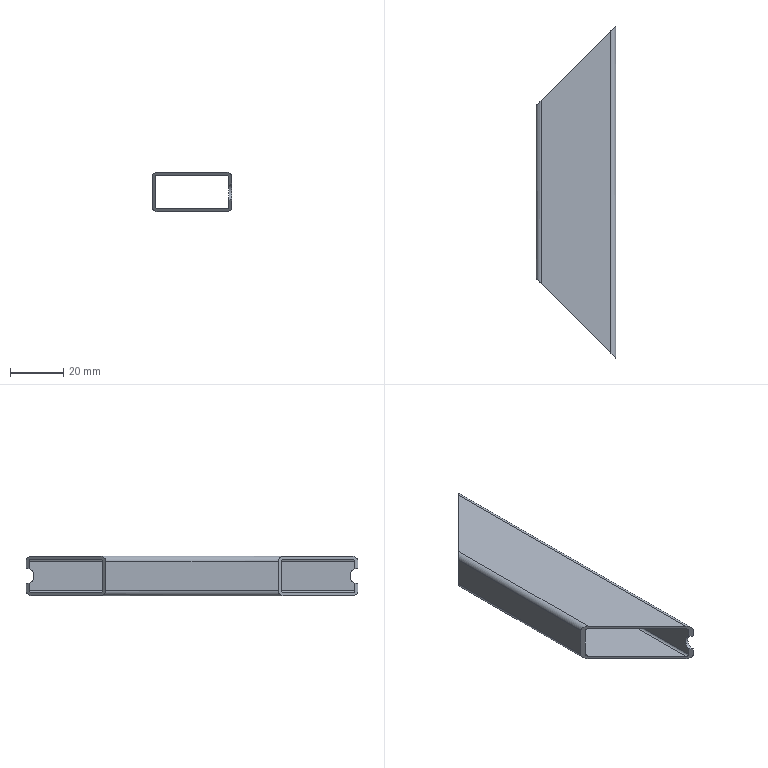Part | STEP file | 6150403 | 1 solid | 20 faces | box 30 x 125 x 15 mm | volume 9413 mm3 | cylinder 10 | plane 10 | commonest cylinder face diameters 1.6 x4 4 x4 6 x2
STEP:
#1=CARTESIAN_POINT('',(-13.,34.5,-7.5));
#2=VERTEX_POINT('',#1);
#3=CARTESIAN_POINT('',(-13.,-34.5,-7.5));
#4=VERTEX_POINT('',#3);
#5=CARTESIAN_POINT('',(-13.,62.5,-7.5));
#6=DIRECTION('',(0.,-1.,0.));
#7=VECTOR('',#6,1000.);
#8=LINE('',#5,#7);
#9=EDGE_CURVE('',#2,#4,#8,.T.);
#10=ORIENTED_EDGE('',*,*,#9,.T.);
#11=CARTESIAN_POINT('',(-15.,-32.5,-5.5));
#12=VERTEX_POINT('',#11);
#13=CARTESIAN_POINT('',(-13.,-34.5,-7.5));
#14=CARTESIAN_POINT('',(-14.172,-33.328,-7.5));
#15=CARTESIAN_POINT('',(-15.,-32.5,-6.672));
#16=CARTESIAN_POINT('',(-15.,-32.5,-5.5));
#17=(BOUNDED_CURVE()B_SPLINE_CURVE(3,(#13,#14,#15,#16),.UNSPECIFIED.,.F.,.F.)B_SPLINE_CURVE_WITH_KNOTS((4,4),(1.571,3.142),.UNSPECIFIED.)CURVE()GEOMETRIC_REPRESENTATION_ITEM()RATIONAL_B_SPLINE_CURVE((1.,0.8047,0.8047,1.))REPRESENTATION_ITEM(''));
#18=EDGE_CURVE('',#4,#12,#17,.T.);
#19=ORIENTED_EDGE('',*,*,#18,.T.);
#20=CARTESIAN_POINT('',(-15.,32.5,-5.5));
#21=VERTEX_POINT('',#20);
#22=CARTESIAN_POINT('',(-15.,62.5,-5.5));
#23=DIRECTION('',(0.,-1.,0.));
#24=VECTOR('',#23,1000.);
#25=LINE('',#22,#24);
#26=EDGE_CURVE('',#21,#12,#25,.T.);
#27=ORIENTED_EDGE('',*,*,#26,.F.);
#28=CARTESIAN_POINT('',(-15.,32.5,-5.5));
#29=CARTESIAN_POINT('',(-15.,32.5,-6.672));
#30=CARTESIAN_POINT('',(-14.172,33.328,-7.5));
#31=CARTESIAN_POINT('',(-13.,34.5,-7.5));
#32=(BOUNDED_CURVE()B_SPLINE_CURVE(3,(#28,#29,#30,#31),.UNSPECIFIED.,.F.,.F.)B_SPLINE_CURVE_WITH_KNOTS((4,4),(0.,1.571),.UNSPECIFIED.)CURVE()GEOMETRIC_REPRESENTATION_ITEM()RATIONAL_B_SPLINE_CURVE((1.,0.8047,0.8047,1.))REPRESENTATION_ITEM(''));
#33=EDGE_CURVE('',#21,#2,#32,.T.);
#34=ORIENTED_EDGE('',*,*,#33,.T.);
#35=EDGE_LOOP('',(#10,#19,#27,#34));
#36=FACE_OUTER_BOUND('',#35,.T.);
#37=CARTESIAN_POINT('',(-13.,62.5,-5.5));
#38=DIRECTION('',(0.,-1.,0.));
#39=DIRECTION('',(0.,0.,-1.));
#40=AXIS2_PLACEMENT_3D('',#37,#38,#39);
#41=CYLINDRICAL_SURFACE('',#40,2.);
#42=ADVANCED_FACE('',(#36),#41,.T.);
#43=ORIENTED_EDGE('',*,*,#26,.T.);
#44=CARTESIAN_POINT('',(-15.,-32.5,5.5));
#45=VERTEX_POINT('',#44);
#46=CARTESIAN_POINT('',(-15.,-32.5,192.5));
#47=DIRECTION('',(0.,0.,-1.));
#48=VECTOR('',#47,1000.);
#49=LINE('',#46,#48);
#50=EDGE_CURVE('',#45,#12,#49,.T.);
#51=ORIENTED_EDGE('',*,*,#50,.F.);
#52=CARTESIAN_POINT('',(-15.,32.5,5.5));
#53=VERTEX_POINT('',#52);
#54=CARTESIAN_POINT('',(-15.,62.5,5.5));
#55=DIRECTION('',(0.,-1.,0.));
#56=VECTOR('',#55,1000.);
#57=LINE('',#54,#56);
#58=EDGE_CURVE('',#53,#45,#57,.T.);
#59=ORIENTED_EDGE('',*,*,#58,.F.);
#60=CARTESIAN_POINT('',(-15.,32.5,192.5));
#61=DIRECTION('',(0.,0.,-1.));
#62=VECTOR('',#61,1000.);
#63=LINE('',#60,#62);
#64=EDGE_CURVE('',#53,#21,#63,.T.);
#65=ORIENTED_EDGE('',*,*,#64,.T.);
#66=EDGE_LOOP('',(#43,#51,#59,#65));
#67=FACE_OUTER_BOUND('',#66,.T.);
#68=CARTESIAN_POINT('',(-15.,62.5,-5.5));
#69=DIRECTION('',(1.,0.,0.));
#70=DIRECTION('',(0.,0.,-1.));
#71=AXIS2_PLACEMENT_3D('',#68,#69,#70);
#72=PLANE('',#71);
#73=ADVANCED_FACE('',(#67),#72,.F.);
#74=ORIENTED_EDGE('',*,*,#58,.T.);
#75=CARTESIAN_POINT('',(-13.,-34.5,7.5));
#76=VERTEX_POINT('',#75);
#77=CARTESIAN_POINT('',(-15.,-32.5,5.5));
#78=CARTESIAN_POINT('',(-15.,-32.5,6.672));
#79=CARTESIAN_POINT('',(-14.172,-33.328,7.5));
#80=CARTESIAN_POINT('',(-13.,-34.5,7.5));
#81=(BOUNDED_CURVE()B_SPLINE_CURVE(3,(#77,#78,#79,#80),.UNSPECIFIED.,.F.,.F.)B_SPLINE_CURVE_WITH_KNOTS((4,4),(3.142,4.712),.UNSPECIFIED.)CURVE()GEOMETRIC_REPRESENTATION_ITEM()RATIONAL_B_SPLINE_CURVE((1.,0.8047,0.8047,1.))REPRESENTATION_ITEM(''));
#82=EDGE_CURVE('',#45,#76,#81,.T.);
#83=ORIENTED_EDGE('',*,*,#82,.T.);
#84=CARTESIAN_POINT('',(-13.,34.5,7.5));
#85=VERTEX_POINT('',#84);
#86=CARTESIAN_POINT('',(-13.,62.5,7.5));
#87=DIRECTION('',(0.,-1.,0.));
#88=VECTOR('',#87,1000.);
#89=LINE('',#86,#88);
#90=EDGE_CURVE('',#85,#76,#89,.T.);
#91=ORIENTED_EDGE('',*,*,#90,.F.);
#92=CARTESIAN_POINT('',(-13.,34.5,7.5));
#93=CARTESIAN_POINT('',(-14.172,33.328,7.5));
#94=CARTESIAN_POINT('',(-15.,32.5,6.672));
#95=CARTESIAN_POINT('',(-15.,32.5,5.5));
#96=(BOUNDED_CURVE()B_SPLINE_CURVE(3,(#92,#93,#94,#95),.UNSPECIFIED.,.F.,.F.)B_SPLINE_CURVE_WITH_KNOTS((4,4),(4.712,6.283),.UNSPECIFIED.)CURVE()GEOMETRIC_REPRESENTATION_ITEM()RATIONAL_B_SPLINE_CURVE((1.,0.8047,0.8047,1.))REPRESENTATION_ITEM(''));
#97=EDGE_CURVE('',#85,#53,#96,.T.);
#98=ORIENTED_EDGE('',*,*,#97,.T.);
#99=EDGE_LOOP('',(#74,#83,#91,#98));
#100=FACE_OUTER_BOUND('',#99,.T.);
#101=CARTESIAN_POINT('',(-13.,62.5,5.5));
#102=DIRECTION('',(0.,-1.,0.));
#103=DIRECTION('',(0.,0.,-1.));
#104=AXIS2_PLACEMENT_3D('',#101,#102,#103);
#105=CYLINDRICAL_SURFACE('',#104,2.);
#106=ADVANCED_FACE('',(#100),#105,.T.);
#107=ORIENTED_EDGE('',*,*,#90,.T.);
#108=CARTESIAN_POINT('',(13.,-60.5,7.5));
#109=VERTEX_POINT('',#108);
#110=CARTESIAN_POINT('',(-61.5,14.,7.5));
#111=DIRECTION('',(0.7071,-0.7071,0.));
#112=VECTOR('',#111,1000.);
#113=LINE('',#110,#112);
#114=EDGE_CURVE('',#76,#109,#113,.T.);
#115=ORIENTED_EDGE('',*,*,#114,.T.);
#116=CARTESIAN_POINT('',(13.,60.5,7.5));
#117=VERTEX_POINT('',#116);
#118=CARTESIAN_POINT('',(13.,62.5,7.5));
#119=DIRECTION('',(0.,-1.,0.));
#120=VECTOR('',#119,1000.);
#121=LINE('',#118,#120);
#122=EDGE_CURVE('',#117,#109,#121,.T.);
#123=ORIENTED_EDGE('',*,*,#122,.F.);
#124=CARTESIAN_POINT('',(1.,48.5,7.5));
#125=DIRECTION('',(-0.7071,-0.7071,0.));
#126=VECTOR('',#125,1000.);
#127=LINE('',#124,#126);
#128=EDGE_CURVE('',#117,#85,#127,.T.);
#129=ORIENTED_EDGE('',*,*,#128,.T.);
#130=EDGE_LOOP('',(#107,#115,#123,#129));
#131=FACE_OUTER_BOUND('',#130,.T.);
#132=CARTESIAN_POINT('',(-13.,62.5,7.5));
#133=DIRECTION('',(0.,0.,-1.));
#134=DIRECTION('',(-1.,0.,0.));
#135=AXIS2_PLACEMENT_3D('',#132,#133,#134);
#136=PLANE('',#135);
#137=ADVANCED_FACE('',(#131),#136,.F.);
#138=ORIENTED_EDGE('',*,*,#122,.T.);
#139=CARTESIAN_POINT('',(15.,-62.5,5.5));
#140=VERTEX_POINT('',#139);
#141=CARTESIAN_POINT('',(13.,-60.5,7.5));
#142=CARTESIAN_POINT('',(14.172,-61.672,7.5));
#143=CARTESIAN_POINT('',(15.,-62.5,6.672));
#144=CARTESIAN_POINT('',(15.,-62.5,5.5));
#145=(BOUNDED_CURVE()B_SPLINE_CURVE(3,(#141,#142,#143,#144),.UNSPECIFIED.,.F.,.F.)B_SPLINE_CURVE_WITH_KNOTS((4,4),(4.712,6.283),.UNSPECIFIED.)CURVE()GEOMETRIC_REPRESENTATION_ITEM()RATIONAL_B_SPLINE_CURVE((1.,0.8047,0.8047,1.))REPRESENTATION_ITEM(''));
#146=EDGE_CURVE('',#109,#140,#145,.T.);
#147=ORIENTED_EDGE('',*,*,#146,.T.);
#148=CARTESIAN_POINT('',(15.,62.5,5.5));
#149=VERTEX_POINT('',#148);
#150=CARTESIAN_POINT('',(15.,62.5,5.5));
#151=DIRECTION('',(0.,-1.,0.));
#152=VECTOR('',#151,1000.);
#153=LINE('',#150,#152);
#154=EDGE_CURVE('',#149,#140,#153,.T.);
#155=ORIENTED_EDGE('',*,*,#154,.F.);
#156=CARTESIAN_POINT('',(15.,62.5,5.5));
#157=CARTESIAN_POINT('',(15.,62.5,6.672));
#158=CARTESIAN_POINT('',(14.172,61.672,7.5));
#159=CARTESIAN_POINT('',(13.,60.5,7.5));
#160=(BOUNDED_CURVE()B_SPLINE_CURVE(3,(#156,#157,#158,#159),.UNSPECIFIED.,.F.,.F.)B_SPLINE_CURVE_WITH_KNOTS((4,4),(3.142,4.712),.UNSPECIFIED.)CURVE()GEOMETRIC_REPRESENTATION_ITEM()RATIONAL_B_SPLINE_CURVE((1.,0.8047,0.8047,1.))REPRESENTATION_ITEM(''));
#161=EDGE_CURVE('',#149,#117,#160,.T.);
#162=ORIENTED_EDGE('',*,*,#161,.T.);
#163=EDGE_LOOP('',(#138,#147,#155,#162));
#164=FACE_OUTER_BOUND('',#163,.T.);
#165=CARTESIAN_POINT('',(13.,62.5,5.5));
#166=DIRECTION('',(0.,-1.,0.));
#167=DIRECTION('',(0.,0.,-1.));
#168=AXIS2_PLACEMENT_3D('',#165,#166,#167);
#169=CYLINDRICAL_SURFACE('',#168,2.);
#170=ADVANCED_FACE('',(#164),#169,.T.);
#171=CARTESIAN_POINT('',(15.,-62.5,3.));
#172=VERTEX_POINT('',#171);
#173=CARTESIAN_POINT('',(15.,-62.5,-5.5));
#174=DIRECTION('',(0.,0.,-1.));
#175=VECTOR('',#174,1000.);
#176=LINE('',#173,#175);
#177=EDGE_CURVE('',#140,#172,#176,.T.);
#178=ORIENTED_EDGE('',*,*,#177,.T.);
#179=CARTESIAN_POINT('',(15.,-62.5,-3.));
#180=VERTEX_POINT('',#179);
#181=CARTESIAN_POINT('',(15.,-62.5,0.));
#182=DIRECTION('',(1.,0.,0.));
#183=DIRECTION('',(0.,0.,-1.));
#184=AXIS2_PLACEMENT_3D('',#181,#182,#183);
#185=CIRCLE('',#184,3.);
#186=EDGE_CURVE('',#180,#172,#185,.T.);
#187=ORIENTED_EDGE('',*,*,#186,.F.);
#188=CARTESIAN_POINT('',(15.,-62.5,-5.5));
#189=VERTEX_POINT('',#188);
#190=CARTESIAN_POINT('',(15.,-62.5,-5.5));
#191=DIRECTION('',(0.,0.,-1.));
#192=VECTOR('',#191,1000.);
#193=LINE('',#190,#192);
#194=EDGE_CURVE('',#180,#189,#193,.T.);
#195=ORIENTED_EDGE('',*,*,#194,.T.);
#196=CARTESIAN_POINT('',(15.,62.5,-5.5));
#197=VERTEX_POINT('',#196);
#198=CARTESIAN_POINT('',(15.,62.5,-5.5));
#199=DIRECTION('',(0.,-1.,0.));
#200=VECTOR('',#199,1000.);
#201=LINE('',#198,#200);
#202=EDGE_CURVE('',#197,#189,#201,.T.);
#203=ORIENTED_EDGE('',*,*,#202,.F.);
#204=CARTESIAN_POINT('',(15.,62.5,-3.));
#205=VERTEX_POINT('',#204);
#206=CARTESIAN_POINT('',(15.,62.5,-5.5));
#207=DIRECTION('',(0.,0.,-1.));
#208=VECTOR('',#207,1000.);
#209=LINE('',#206,#208);
#210=EDGE_CURVE('',#205,#197,#209,.T.);
#211=ORIENTED_EDGE('',*,*,#210,.F.);
#212=CARTESIAN_POINT('',(15.,62.5,3.));
#213=VERTEX_POINT('',#212);
#214=CARTESIAN_POINT('',(15.,62.5,0.));
#215=DIRECTION('',(1.,0.,0.));
#216=DIRECTION('',(0.,0.,-1.));
#217=AXIS2_PLACEMENT_3D('',#214,#215,#216);
#218=CIRCLE('',#217,3.);
#219=EDGE_CURVE('',#213,#205,#218,.T.);
#220=ORIENTED_EDGE('',*,*,#219,.F.);
#221=CARTESIAN_POINT('',(15.,62.5,-5.5));
#222=DIRECTION('',(0.,0.,-1.));
#223=VECTOR('',#222,1000.);
#224=LINE('',#221,#223);
#225=EDGE_CURVE('',#149,#213,#224,.T.);
#226=ORIENTED_EDGE('',*,*,#225,.F.);
#227=ORIENTED_EDGE('',*,*,#154,.T.);
#228=EDGE_LOOP('',(#178,#187,#195,#203,#211,#220,#226,#227));
#229=FACE_OUTER_BOUND('',#228,.T.);
#230=CARTESIAN_POINT('',(15.,62.5,-5.5));
#231=DIRECTION('',(-1.,0.,0.));
#232=DIRECTION('',(0.,0.,1.));
#233=AXIS2_PLACEMENT_3D('',#230,#231,#232);
#234=PLANE('',#233);
#235=ADVANCED_FACE('',(#229),#234,.F.);
#236=ORIENTED_EDGE('',*,*,#202,.T.);
#237=CARTESIAN_POINT('',(13.,-60.5,-7.5));
#238=VERTEX_POINT('',#237);
#239=CARTESIAN_POINT('',(15.,-62.5,-5.5));
#240=CARTESIAN_POINT('',(15.,-62.5,-6.672));
#241=CARTESIAN_POINT('',(14.172,-61.672,-7.5));
#242=CARTESIAN_POINT('',(13.,-60.5,-7.5));
#243=(BOUNDED_CURVE()B_SPLINE_CURVE(3,(#239,#240,#241,#242),.UNSPECIFIED.,.F.,.F.)B_SPLINE_CURVE_WITH_KNOTS((4,4),(0.,1.571),.UNSPECIFIED.)CURVE()GEOMETRIC_REPRESENTATION_ITEM()RATIONAL_B_SPLINE_CURVE((1.,0.8047,0.8047,1.))REPRESENTATION_ITEM(''));
#244=EDGE_CURVE('',#189,#238,#243,.T.);
#245=ORIENTED_EDGE('',*,*,#244,.T.);
#246=CARTESIAN_POINT('',(13.,60.5,-7.5));
#247=VERTEX_POINT('',#246);
#248=CARTESIAN_POINT('',(13.,62.5,-7.5));
#249=DIRECTION('',(0.,-1.,0.));
#250=VECTOR('',#249,1000.);
#251=LINE('',#248,#250);
#252=EDGE_CURVE('',#247,#238,#251,.T.);
#253=ORIENTED_EDGE('',*,*,#252,.F.);
#254=CARTESIAN_POINT('',(13.,60.5,-7.5));
#255=CARTESIAN_POINT('',(14.172,61.672,-7.5));
#256=CARTESIAN_POINT('',(15.,62.5,-6.672));
#257=CARTESIAN_POINT('',(15.,62.5,-5.5));
#258=(BOUNDED_CURVE()B_SPLINE_CURVE(3,(#254,#255,#256,#257),.UNSPECIFIED.,.F.,.F.)B_SPLINE_CURVE_WITH_KNOTS((4,4),(1.571,3.142),.UNSPECIFIED.)CURVE()GEOMETRIC_REPRESENTATION_ITEM()RATIONAL_B_SPLINE_CURVE((1.,0.8047,0.8047,1.))REPRESENTATION_ITEM(''));
#259=EDGE_CURVE('',#247,#197,#258,.T.);
#260=ORIENTED_EDGE('',*,*,#259,.T.);
#261=EDGE_LOOP('',(#236,#245,#253,#260));
#262=FACE_OUTER_BOUND('',#261,.T.);
#263=CARTESIAN_POINT('',(13.,62.5,-5.5));
#264=DIRECTION('',(0.,-1.,0.));
#265=DIRECTION('',(0.,0.,-1.));
#266=AXIS2_PLACEMENT_3D('',#263,#264,#265);
#267=CYLINDRICAL_SURFACE('',#266,2.);
#268=ADVANCED_FACE('',(#262),#267,.T.);
#269=ORIENTED_EDGE('',*,*,#252,.T.);
#270=CARTESIAN_POINT('',(15.,-62.5,-7.5));
#271=DIRECTION('',(0.7071,-0.7071,0.));
#272=VECTOR('',#271,1000.);
#273=LINE('',#270,#272);
#274=EDGE_CURVE('',#4,#238,#273,.T.);
#275=ORIENTED_EDGE('',*,*,#274,.F.);
#276=ORIENTED_EDGE('',*,*,#9,.F.);
#277=CARTESIAN_POINT('',(15.,62.5,-7.5));
#278=DIRECTION('',(-0.7071,-0.7071,0.));
#279=VECTOR('',#278,1000.);
#280=LINE('',#277,#279);
#281=EDGE_CURVE('',#247,#2,#280,.T.);
#282=ORIENTED_EDGE('',*,*,#281,.F.);
#283=EDGE_LOOP('',(#269,#275,#276,#282));
#284=FACE_OUTER_BOUND('',#283,.T.);
#285=CARTESIAN_POINT('',(-13.,62.5,-7.5));
#286=DIRECTION('',(0.,0.,1.));
#287=DIRECTION('',(1.,0.,0.));
#288=AXIS2_PLACEMENT_3D('',#285,#286,#287);
#289=PLANE('',#288);
#290=ADVANCED_FACE('',(#284),#289,.F.);
#291=CARTESIAN_POINT('',(13.8,-61.3,-5.5));
#292=VERTEX_POINT('',#291);
#293=CARTESIAN_POINT('',(13.,-60.5,-6.3));
#294=VERTEX_POINT('',#293);
#295=CARTESIAN_POINT('',(13.8,-61.3,-5.5));
#296=CARTESIAN_POINT('',(13.8,-61.3,-5.969));
#297=CARTESIAN_POINT('',(13.469,-60.969,-6.3));
#298=CARTESIAN_POINT('',(13.,-60.5,-6.3));
#299=(BOUNDED_CURVE()B_SPLINE_CURVE(3,(#295,#296,#297,#298),.UNSPECIFIED.,.F.,.F.)B_SPLINE_CURVE_WITH_KNOTS((4,4),(0.,1.571),.UNSPECIFIED.)CURVE()GEOMETRIC_REPRESENTATION_ITEM()RATIONAL_B_SPLINE_CURVE((1.,0.8047,0.8047,1.))REPRESENTATION_ITEM(''));
#300=EDGE_CURVE('',#292,#294,#299,.T.);
#301=ORIENTED_EDGE('',*,*,#300,.F.);
#302=CARTESIAN_POINT('',(13.8,61.3,-5.5));
#303=VERTEX_POINT('',#302);
#304=CARTESIAN_POINT('',(13.8,62.5,-5.5));
#305=DIRECTION('',(0.,-1.,0.));
#306=VECTOR('',#305,1000.);
#307=LINE('',#304,#306);
#308=EDGE_CURVE('',#303,#292,#307,.T.);
#309=ORIENTED_EDGE('',*,*,#308,.F.);
#310=CARTESIAN_POINT('',(13.,60.5,-6.3));
#311=VERTEX_POINT('',#310);
#312=CARTESIAN_POINT('',(13.,60.5,-6.3));
#313=CARTESIAN_POINT('',(13.469,60.969,-6.3));
#314=CARTESIAN_POINT('',(13.8,61.3,-5.969));
#315=CARTESIAN_POINT('',(13.8,61.3,-5.5));
#316=(BOUNDED_CURVE()B_SPLINE_CURVE(3,(#312,#313,#314,#315),.UNSPECIFIED.,.F.,.F.)B_SPLINE_CURVE_WITH_KNOTS((4,4),(1.571,3.142),.UNSPECIFIED.)CURVE()GEOMETRIC_REPRESENTATION_ITEM()RATIONAL_B_SPLINE_CURVE((1.,0.8047,0.8047,1.))REPRESENTATION_ITEM(''));
#317=EDGE_CURVE('',#311,#303,#316,.T.);
#318=ORIENTED_EDGE('',*,*,#317,.F.);
#319=CARTESIAN_POINT('',(13.,62.5,-6.3));
#320=DIRECTION('',(0.,-1.,0.));
#321=VECTOR('',#320,1000.);
#322=LINE('',#319,#321);
#323=EDGE_CURVE('',#311,#294,#322,.T.);
#324=ORIENTED_EDGE('',*,*,#323,.T.);
#325=EDGE_LOOP('',(#301,#309,#318,#324));
#326=FACE_OUTER_BOUND('',#325,.T.);
#327=CARTESIAN_POINT('',(13.,62.5,-5.5));
#328=DIRECTION('',(0.,-1.,0.));
#329=DIRECTION('',(0.,0.,-1.));
#330=AXIS2_PLACEMENT_3D('',#327,#328,#329);
#331=CYLINDRICAL_SURFACE('',#330,0.8);
#332=ADVANCED_FACE('',(#326),#331,.F.);
#333=CARTESIAN_POINT('',(-13.,-34.5,-6.3));
#334=VERTEX_POINT('',#333);
#335=CARTESIAN_POINT('',(-61.5,14.,-6.3));
#336=DIRECTION('',(-0.7071,0.7071,0.));
#337=VECTOR('',#336,1000.);
#338=LINE('',#335,#337);
#339=EDGE_CURVE('',#294,#334,#338,.T.);
#340=ORIENTED_EDGE('',*,*,#339,.F.);
#341=ORIENTED_EDGE('',*,*,#323,.F.);
#342=CARTESIAN_POINT('',(-13.,34.5,-6.3));
#343=VERTEX_POINT('',#342);
#344=CARTESIAN_POINT('',(1.,48.5,-6.3));
#345=DIRECTION('',(0.7071,0.7071,0.));
#346=VECTOR('',#345,1000.);
#347=LINE('',#344,#346);
#348=EDGE_CURVE('',#343,#311,#347,.T.);
#349=ORIENTED_EDGE('',*,*,#348,.F.);
#350=CARTESIAN_POINT('',(-13.,62.5,-6.3));
#351=DIRECTION('',(0.,-1.,0.));
#352=VECTOR('',#351,1000.);
#353=LINE('',#350,#352);
#354=EDGE_CURVE('',#343,#334,#353,.T.);
#355=ORIENTED_EDGE('',*,*,#354,.T.);
#356=EDGE_LOOP('',(#340,#341,#349,#355));
#357=FACE_OUTER_BOUND('',#356,.T.);
#358=CARTESIAN_POINT('',(-13.,62.5,-6.3));
#359=DIRECTION('',(0.,0.,1.));
#360=DIRECTION('',(1.,0.,0.));
#361=AXIS2_PLACEMENT_3D('',#358,#359,#360);
#362=PLANE('',#361);
#363=ADVANCED_FACE('',(#357),#362,.T.);
#364=CARTESIAN_POINT('',(-13.8,-33.7,-5.5));
#365=VERTEX_POINT('',#364);
#366=CARTESIAN_POINT('',(-13.,-34.5,-6.3));
#367=CARTESIAN_POINT('',(-13.469,-34.031,-6.3));
#368=CARTESIAN_POINT('',(-13.8,-33.7,-5.969));
#369=CARTESIAN_POINT('',(-13.8,-33.7,-5.5));
#370=(BOUNDED_CURVE()B_SPLINE_CURVE(3,(#366,#367,#368,#369),.UNSPECIFIED.,.F.,.F.)B_SPLINE_CURVE_WITH_KNOTS((4,4),(1.571,3.142),.UNSPECIFIED.)CURVE()GEOMETRIC_REPRESENTATION_ITEM()RATIONAL_B_SPLINE_CURVE((1.,0.8047,0.8047,1.))REPRESENTATION_ITEM(''));
#371=EDGE_CURVE('',#334,#365,#370,.T.);
#372=ORIENTED_EDGE('',*,*,#371,.F.);
#373=ORIENTED_EDGE('',*,*,#354,.F.);
#374=CARTESIAN_POINT('',(-13.8,33.7,-5.5));
#375=VERTEX_POINT('',#374);
#376=CARTESIAN_POINT('',(-13.8,33.7,-5.5));
#377=CARTESIAN_POINT('',(-13.8,33.7,-5.969));
#378=CARTESIAN_POINT('',(-13.469,34.031,-6.3));
#379=CARTESIAN_POINT('',(-13.,34.5,-6.3));
#380=(BOUNDED_CURVE()B_SPLINE_CURVE(3,(#376,#377,#378,#379),.UNSPECIFIED.,.F.,.F.)B_SPLINE_CURVE_WITH_KNOTS((4,4),(0.,1.571),.UNSPECIFIED.)CURVE()GEOMETRIC_REPRESENTATION_ITEM()RATIONAL_B_SPLINE_CURVE((1.,0.8047,0.8047,1.))REPRESENTATION_ITEM(''));
#381=EDGE_CURVE('',#375,#343,#380,.T.);
#382=ORIENTED_EDGE('',*,*,#381,.F.);
#383=CARTESIAN_POINT('',(-13.8,62.5,-5.5));
#384=DIRECTION('',(0.,-1.,0.));
#385=VECTOR('',#384,1000.);
#386=LINE('',#383,#385);
#387=EDGE_CURVE('',#375,#365,#386,.T.);
#388=ORIENTED_EDGE('',*,*,#387,.T.);
#389=EDGE_LOOP('',(#372,#373,#382,#388));
#390=FACE_OUTER_BOUND('',#389,.T.);
#391=CARTESIAN_POINT('',(-13.,62.5,-5.5));
#392=DIRECTION('',(0.,-1.,0.));
#393=DIRECTION('',(0.,0.,-1.));
#394=AXIS2_PLACEMENT_3D('',#391,#392,#393);
#395=CYLINDRICAL_SURFACE('',#394,0.8);
#396=ADVANCED_FACE('',(#390),#395,.F.);
#397=CARTESIAN_POINT('',(-13.8,-33.7,5.5));
#398=VERTEX_POINT('',#397);
#399=CARTESIAN_POINT('',(-13.8,-33.7,-5.5));
#400=DIRECTION('',(0.,0.,1.));
#401=VECTOR('',#400,1000.);
#402=LINE('',#399,#401);
#403=EDGE_CURVE('',#365,#398,#402,.T.);
#404=ORIENTED_EDGE('',*,*,#403,.F.);
#405=ORIENTED_EDGE('',*,*,#387,.F.);
#406=CARTESIAN_POINT('',(-13.8,33.7,5.5));
#407=VERTEX_POINT('',#406);
#408=CARTESIAN_POINT('',(-13.8,33.7,-5.5));
#409=DIRECTION('',(0.,0.,-1.));
#410=VECTOR('',#409,1000.);
#411=LINE('',#408,#410);
#412=EDGE_CURVE('',#407,#375,#411,.T.);
#413=ORIENTED_EDGE('',*,*,#412,.F.);
#414=CARTESIAN_POINT('',(-13.8,62.5,5.5));
#415=DIRECTION('',(0.,-1.,0.));
#416=VECTOR('',#415,1000.);
#417=LINE('',#414,#416);
#418=EDGE_CURVE('',#407,#398,#417,.T.);
#419=ORIENTED_EDGE('',*,*,#418,.T.);
#420=EDGE_LOOP('',(#404,#405,#413,#419));
#421=FACE_OUTER_BOUND('',#420,.T.);
#422=CARTESIAN_POINT('',(-13.8,62.5,-5.5));
#423=DIRECTION('',(1.,0.,0.));
#424=DIRECTION('',(0.,0.,-1.));
#425=AXIS2_PLACEMENT_3D('',#422,#423,#424);
#426=PLANE('',#425);
#427=ADVANCED_FACE('',(#421),#426,.T.);
#428=CARTESIAN_POINT('',(-13.,-34.5,6.3));
#429=VERTEX_POINT('',#428);
#430=CARTESIAN_POINT('',(-13.8,-33.7,5.5));
#431=CARTESIAN_POINT('',(-13.8,-33.7,5.969));
#432=CARTESIAN_POINT('',(-13.469,-34.031,6.3));
#433=CARTESIAN_POINT('',(-13.,-34.5,6.3));
#434=(BOUNDED_CURVE()B_SPLINE_CURVE(3,(#430,#431,#432,#433),.UNSPECIFIED.,.F.,.F.)B_SPLINE_CURVE_WITH_KNOTS((4,4),(3.142,4.712),.UNSPECIFIED.)CURVE()GEOMETRIC_REPRESENTATION_ITEM()RATIONAL_B_SPLINE_CURVE((1.,0.8047,0.8047,1.))REPRESENTATION_ITEM(''));
#435=EDGE_CURVE('',#398,#429,#434,.T.);
#436=ORIENTED_EDGE('',*,*,#435,.F.);
#437=ORIENTED_EDGE('',*,*,#418,.F.);
#438=CARTESIAN_POINT('',(-13.,34.5,6.3));
#439=VERTEX_POINT('',#438);
#440=CARTESIAN_POINT('',(-13.,34.5,6.3));
#441=CARTESIAN_POINT('',(-13.469,34.031,6.3));
#442=CARTESIAN_POINT('',(-13.8,33.7,5.969));
#443=CARTESIAN_POINT('',(-13.8,33.7,5.5));
#444=(BOUNDED_CURVE()B_SPLINE_CURVE(3,(#440,#441,#442,#443),.UNSPECIFIED.,.F.,.F.)B_SPLINE_CURVE_WITH_KNOTS((4,4),(4.712,6.283),.UNSPECIFIED.)CURVE()GEOMETRIC_REPRESENTATION_ITEM()RATIONAL_B_SPLINE_CURVE((1.,0.8047,0.8047,1.))REPRESENTATION_ITEM(''));
#445=EDGE_CURVE('',#439,#407,#444,.T.);
#446=ORIENTED_EDGE('',*,*,#445,.F.);
#447=CARTESIAN_POINT('',(-13.,62.5,6.3));
#448=DIRECTION('',(0.,-1.,0.));
#449=VECTOR('',#448,1000.);
#450=LINE('',#447,#449);
#451=EDGE_CURVE('',#439,#429,#450,.T.);
#452=ORIENTED_EDGE('',*,*,#451,.T.);
#453=EDGE_LOOP('',(#436,#437,#446,#452));
#454=FACE_OUTER_BOUND('',#453,.T.);
#455=CARTESIAN_POINT('',(-13.,62.5,5.5));
#456=DIRECTION('',(0.,-1.,0.));
#457=DIRECTION('',(0.,0.,-1.));
#458=AXIS2_PLACEMENT_3D('',#455,#456,#457);
#459=CYLINDRICAL_SURFACE('',#458,0.8);
#460=ADVANCED_FACE('',(#454),#459,.F.);
#461=CARTESIAN_POINT('',(13.,-60.5,6.3));
#462=VERTEX_POINT('',#461);
#463=CARTESIAN_POINT('',(-61.5,14.,6.3));
#464=DIRECTION('',(0.7071,-0.7071,0.));
#465=VECTOR('',#464,1000.);
#466=LINE('',#463,#465);
#467=EDGE_CURVE('',#429,#462,#466,.T.);
#468=ORIENTED_EDGE('',*,*,#467,.F.);
#469=ORIENTED_EDGE('',*,*,#451,.F.);
#470=CARTESIAN_POINT('',(13.,60.5,6.3));
#471=VERTEX_POINT('',#470);
#472=CARTESIAN_POINT('',(1.,48.5,6.3));
#473=DIRECTION('',(-0.7071,-0.7071,0.));
#474=VECTOR('',#473,1000.);
#475=LINE('',#472,#474);
#476=EDGE_CURVE('',#471,#439,#475,.T.);
#477=ORIENTED_EDGE('',*,*,#476,.F.);
#478=CARTESIAN_POINT('',(13.,62.5,6.3));
#479=DIRECTION('',(0.,-1.,0.));
#480=VECTOR('',#479,1000.);
#481=LINE('',#478,#480);
#482=EDGE_CURVE('',#471,#462,#481,.T.);
#483=ORIENTED_EDGE('',*,*,#482,.T.);
#484=EDGE_LOOP('',(#468,#469,#477,#483));
#485=FACE_OUTER_BOUND('',#484,.T.);
#486=CARTESIAN_POINT('',(-13.,62.5,6.3));
#487=DIRECTION('',(0.,0.,-1.));
#488=DIRECTION('',(-1.,0.,0.));
#489=AXIS2_PLACEMENT_3D('',#486,#487,#488);
#490=PLANE('',#489);
#491=ADVANCED_FACE('',(#485),#490,.T.);
#492=CARTESIAN_POINT('',(13.8,-61.3,5.5));
#493=VERTEX_POINT('',#492);
#494=CARTESIAN_POINT('',(13.,-60.5,6.3));
#495=CARTESIAN_POINT('',(13.469,-60.969,6.3));
#496=CARTESIAN_POINT('',(13.8,-61.3,5.969));
#497=CARTESIAN_POINT('',(13.8,-61.3,5.5));
#498=(BOUNDED_CURVE()B_SPLINE_CURVE(3,(#494,#495,#496,#497),.UNSPECIFIED.,.F.,.F.)B_SPLINE_CURVE_WITH_KNOTS((4,4),(4.712,6.283),.UNSPECIFIED.)CURVE()GEOMETRIC_REPRESENTATION_ITEM()RATIONAL_B_SPLINE_CURVE((1.,0.8047,0.8047,1.))REPRESENTATION_ITEM(''));
#499=EDGE_CURVE('',#462,#493,#498,.T.);
#500=ORIENTED_EDGE('',*,*,#499,.F.);
#501=ORIENTED_EDGE('',*,*,#482,.F.);
#502=CARTESIAN_POINT('',(13.8,61.3,5.5));
#503=VERTEX_POINT('',#502);
#504=CARTESIAN_POINT('',(13.8,61.3,5.5));
#505=CARTESIAN_POINT('',(13.8,61.3,5.969));
#506=CARTESIAN_POINT('',(13.469,60.969,6.3));
#507=CARTESIAN_POINT('',(13.,60.5,6.3));
#508=(BOUNDED_CURVE()B_SPLINE_CURVE(3,(#504,#505,#506,#507),.UNSPECIFIED.,.F.,.F.)B_SPLINE_CURVE_WITH_KNOTS((4,4),(3.142,4.712),.UNSPECIFIED.)CURVE()GEOMETRIC_REPRESENTATION_ITEM()RATIONAL_B_SPLINE_CURVE((1.,0.8047,0.8047,1.))REPRESENTATION_ITEM(''));
#509=EDGE_CURVE('',#503,#471,#508,.T.);
#510=ORIENTED_EDGE('',*,*,#509,.F.);
#511=CARTESIAN_POINT('',(13.8,62.5,5.5));
#512=DIRECTION('',(0.,-1.,0.));
#513=VECTOR('',#512,1000.);
#514=LINE('',#511,#513);
#515=EDGE_CURVE('',#503,#493,#514,.T.);
#516=ORIENTED_EDGE('',*,*,#515,.T.);
#517=EDGE_LOOP('',(#500,#501,#510,#516));
#518=FACE_OUTER_BOUND('',#517,.T.);
#519=CARTESIAN_POINT('',(13.,62.5,5.5));
#520=DIRECTION('',(0.,-1.,0.));
#521=DIRECTION('',(0.,0.,-1.));
#522=AXIS2_PLACEMENT_3D('',#519,#520,#521);
#523=CYLINDRICAL_SURFACE('',#522,0.8);
#524=ADVANCED_FACE('',(#518),#523,.F.);
#525=CARTESIAN_POINT('',(13.8,-61.3,2.75));
#526=VERTEX_POINT('',#525);
#527=CARTESIAN_POINT('',(13.8,-61.3,-2.75));
#528=VERTEX_POINT('',#527);
#529=CARTESIAN_POINT('',(13.8,-62.5,0.));
#530=DIRECTION('',(-1.,0.,0.));
#531=DIRECTION('',(0.,0.,1.));
#532=AXIS2_PLACEMENT_3D('',#529,#530,#531);
#533=CIRCLE('',#532,3.);
#534=EDGE_CURVE('',#526,#528,#533,.T.);
#535=ORIENTED_EDGE('',*,*,#534,.F.);
#536=CARTESIAN_POINT('',(13.8,-61.3,-5.5));
#537=DIRECTION('',(0.,0.,-1.));
#538=VECTOR('',#537,1000.);
#539=LINE('',#536,#538);
#540=EDGE_CURVE('',#493,#526,#539,.T.);
#541=ORIENTED_EDGE('',*,*,#540,.F.);
#542=ORIENTED_EDGE('',*,*,#515,.F.);
#543=CARTESIAN_POINT('',(13.8,61.3,2.75));
#544=VERTEX_POINT('',#543);
#545=CARTESIAN_POINT('',(13.8,61.3,-5.5));
#546=DIRECTION('',(0.,0.,1.));
#547=VECTOR('',#546,1000.);
#548=LINE('',#545,#547);
#549=EDGE_CURVE('',#544,#503,#548,.T.);
#550=ORIENTED_EDGE('',*,*,#549,.F.);
#551=CARTESIAN_POINT('',(13.8,61.3,-2.75));
#552=VERTEX_POINT('',#551);
#553=CARTESIAN_POINT('',(13.8,62.5,0.));
#554=DIRECTION('',(-1.,0.,0.));
#555=DIRECTION('',(0.,0.,1.));
#556=AXIS2_PLACEMENT_3D('',#553,#554,#555);
#557=CIRCLE('',#556,3.);
#558=EDGE_CURVE('',#552,#544,#557,.T.);
#559=ORIENTED_EDGE('',*,*,#558,.F.);
#560=CARTESIAN_POINT('',(13.8,61.3,-5.5));
#561=DIRECTION('',(0.,0.,1.));
#562=VECTOR('',#561,1000.);
#563=LINE('',#560,#562);
#564=EDGE_CURVE('',#303,#552,#563,.T.);
#565=ORIENTED_EDGE('',*,*,#564,.F.);
#566=ORIENTED_EDGE('',*,*,#308,.T.);
#567=CARTESIAN_POINT('',(13.8,-61.3,-5.5));
#568=DIRECTION('',(0.,0.,-1.));
#569=VECTOR('',#568,1000.);
#570=LINE('',#567,#569);
#571=EDGE_CURVE('',#528,#292,#570,.T.);
#572=ORIENTED_EDGE('',*,*,#571,.F.);
#573=EDGE_LOOP('',(#535,#541,#542,#550,#559,#565,#566,#572));
#574=FACE_OUTER_BOUND('',#573,.T.);
#575=CARTESIAN_POINT('',(13.8,62.5,-5.5));
#576=DIRECTION('',(-1.,0.,0.));
#577=DIRECTION('',(0.,0.,1.));
#578=AXIS2_PLACEMENT_3D('',#575,#576,#577);
#579=PLANE('',#578);
#580=ADVANCED_FACE('',(#574),#579,.T.);
#581=ORIENTED_EDGE('',*,*,#225,.T.);
#582=CARTESIAN_POINT('',(15.,62.5,3.));
#583=CARTESIAN_POINT('',(14.586,62.086,3.));
#584=CARTESIAN_POINT('',(14.18,61.68,2.915));
#585=CARTESIAN_POINT('',(13.8,61.3,2.75));
#586=(BOUNDED_CURVE()B_SPLINE_CURVE(3,(#582,#583,#584,#585),.UNSPECIFIED.,.F.,.F.)B_SPLINE_CURVE_WITH_KNOTS((4,4),(1.571,1.982),.UNSPECIFIED.)CURVE()GEOMETRIC_REPRESENTATION_ITEM()RATIONAL_B_SPLINE_CURVE((1.,0.9859,0.9859,1.))REPRESENTATION_ITEM(''));
#587=EDGE_CURVE('',#213,#544,#586,.T.);
#588=ORIENTED_EDGE('',*,*,#587,.T.);
#589=ORIENTED_EDGE('',*,*,#549,.T.);
#590=ORIENTED_EDGE('',*,*,#509,.T.);
#591=ORIENTED_EDGE('',*,*,#476,.T.);
#592=ORIENTED_EDGE('',*,*,#445,.T.);
#593=ORIENTED_EDGE('',*,*,#412,.T.);
#594=ORIENTED_EDGE('',*,*,#381,.T.);
#595=ORIENTED_EDGE('',*,*,#348,.T.);
#596=ORIENTED_EDGE('',*,*,#317,.T.);
#597=ORIENTED_EDGE('',*,*,#564,.T.);
#598=CARTESIAN_POINT('',(13.8,61.3,-2.75));
#599=CARTESIAN_POINT('',(14.18,61.68,-2.915));
#600=CARTESIAN_POINT('',(14.586,62.086,-3.));
#601=CARTESIAN_POINT('',(15.,62.5,-3.));
#602=(BOUNDED_CURVE()B_SPLINE_CURVE(3,(#598,#599,#600,#601),.UNSPECIFIED.,.F.,.F.)B_SPLINE_CURVE_WITH_KNOTS((4,4),(4.301,4.712),.UNSPECIFIED.)CURVE()GEOMETRIC_REPRESENTATION_ITEM()RATIONAL_B_SPLINE_CURVE((1.,0.9859,0.9859,1.))REPRESENTATION_ITEM(''));
#603=EDGE_CURVE('',#552,#205,#602,.T.);
#604=ORIENTED_EDGE('',*,*,#603,.T.);
#605=ORIENTED_EDGE('',*,*,#210,.T.);
#606=ORIENTED_EDGE('',*,*,#259,.F.);
#607=ORIENTED_EDGE('',*,*,#281,.T.);
#608=ORIENTED_EDGE('',*,*,#33,.F.);
#609=ORIENTED_EDGE('',*,*,#64,.F.);
#610=ORIENTED_EDGE('',*,*,#97,.F.);
#611=ORIENTED_EDGE('',*,*,#128,.F.);
#612=ORIENTED_EDGE('',*,*,#161,.F.);
#613=EDGE_LOOP('',(#581,#588,#589,#590,#591,#592,#593,#594,#595,#596,#597,#604,#605,#606,#607,#608,#609,#610,#611,#612));
#614=FACE_OUTER_BOUND('',#613,.T.);
#615=CARTESIAN_POINT('',(15.,62.5,192.5));
#616=DIRECTION('',(0.7071,-0.7071,0.));
#617=DIRECTION('',(0.7071,0.7071,0.));
#618=AXIS2_PLACEMENT_3D('',#615,#616,#617);
#619=PLANE('',#618);
#620=ADVANCED_FACE('',(#614),#619,.F.);
#621=ORIENTED_EDGE('',*,*,#194,.F.);
#622=CARTESIAN_POINT('',(15.,-62.5,-3.));
#623=CARTESIAN_POINT('',(14.586,-62.086,-3.));
#624=CARTESIAN_POINT('',(14.18,-61.68,-2.915));
#625=CARTESIAN_POINT('',(13.8,-61.3,-2.75));
#626=(BOUNDED_CURVE()B_SPLINE_CURVE(3,(#622,#623,#624,#625),.UNSPECIFIED.,.F.,.F.)B_SPLINE_CURVE_WITH_KNOTS((4,4),(1.571,1.982),.UNSPECIFIED.)CURVE()GEOMETRIC_REPRESENTATION_ITEM()RATIONAL_B_SPLINE_CURVE((1.,0.9859,0.9859,1.))REPRESENTATION_ITEM(''));
#627=EDGE_CURVE('',#180,#528,#626,.T.);
#628=ORIENTED_EDGE('',*,*,#627,.T.);
#629=ORIENTED_EDGE('',*,*,#571,.T.);
#630=ORIENTED_EDGE('',*,*,#300,.T.);
#631=ORIENTED_EDGE('',*,*,#339,.T.);
#632=ORIENTED_EDGE('',*,*,#371,.T.);
#633=ORIENTED_EDGE('',*,*,#403,.T.);
#634=ORIENTED_EDGE('',*,*,#435,.T.);
#635=ORIENTED_EDGE('',*,*,#467,.T.);
#636=ORIENTED_EDGE('',*,*,#499,.T.);
#637=ORIENTED_EDGE('',*,*,#540,.T.);
#638=CARTESIAN_POINT('',(13.8,-61.3,2.75));
#639=CARTESIAN_POINT('',(14.18,-61.68,2.915));
#640=CARTESIAN_POINT('',(14.586,-62.086,3.));
#641=CARTESIAN_POINT('',(15.,-62.5,3.));
#642=(BOUNDED_CURVE()B_SPLINE_CURVE(3,(#638,#639,#640,#641),.UNSPECIFIED.,.F.,.F.)B_SPLINE_CURVE_WITH_KNOTS((4,4),(4.301,4.712),.UNSPECIFIED.)CURVE()GEOMETRIC_REPRESENTATION_ITEM()RATIONAL_B_SPLINE_CURVE((1.,0.9859,0.9859,1.))REPRESENTATION_ITEM(''));
#643=EDGE_CURVE('',#526,#172,#642,.T.);
#644=ORIENTED_EDGE('',*,*,#643,.T.);
#645=ORIENTED_EDGE('',*,*,#177,.F.);
#646=ORIENTED_EDGE('',*,*,#146,.F.);
#647=ORIENTED_EDGE('',*,*,#114,.F.);
#648=ORIENTED_EDGE('',*,*,#82,.F.);
#649=ORIENTED_EDGE('',*,*,#50,.T.);
#650=ORIENTED_EDGE('',*,*,#18,.F.);
#651=ORIENTED_EDGE('',*,*,#274,.T.);
#652=ORIENTED_EDGE('',*,*,#244,.F.);
#653=EDGE_LOOP('',(#621,#628,#629,#630,#631,#632,#633,#634,#635,#636,#637,#644,#645,#646,#647,#648,#649,#650,#651,#652));
#654=FACE_OUTER_BOUND('',#653,.T.);
#655=CARTESIAN_POINT('',(15.,-62.5,192.5));
#656=DIRECTION('',(0.7071,0.7071,0.));
#657=DIRECTION('',(-0.7071,0.7071,0.));
#658=AXIS2_PLACEMENT_3D('',#655,#656,#657);
#659=PLANE('',#658);
#660=ADVANCED_FACE('',(#654),#659,.F.);
#661=ORIENTED_EDGE('',*,*,#219,.T.);
#662=ORIENTED_EDGE('',*,*,#603,.F.);
#663=ORIENTED_EDGE('',*,*,#558,.T.);
#664=ORIENTED_EDGE('',*,*,#587,.F.);
#665=EDGE_LOOP('',(#661,#662,#663,#664));
#666=FACE_OUTER_BOUND('',#665,.T.);
#667=CARTESIAN_POINT('',(5.,62.5,0.));
#668=DIRECTION('',(1.,0.,0.));
#669=DIRECTION('',(0.,0.,-1.));
#670=AXIS2_PLACEMENT_3D('',#667,#668,#669);
#671=CYLINDRICAL_SURFACE('',#670,3.);
#672=ADVANCED_FACE('',(#666),#671,.F.);
#673=ORIENTED_EDGE('',*,*,#186,.T.);
#674=ORIENTED_EDGE('',*,*,#643,.F.);
#675=ORIENTED_EDGE('',*,*,#534,.T.);
#676=ORIENTED_EDGE('',*,*,#627,.F.);
#677=EDGE_LOOP('',(#673,#674,#675,#676));
#678=FACE_OUTER_BOUND('',#677,.T.);
#679=CARTESIAN_POINT('',(5.,-62.5,0.));
#680=DIRECTION('',(1.,0.,0.));
#681=DIRECTION('',(0.,0.,-1.));
#682=AXIS2_PLACEMENT_3D('',#679,#680,#681);
#683=CYLINDRICAL_SURFACE('',#682,3.);
#684=ADVANCED_FACE('',(#678),#683,.F.);
#685=CLOSED_SHELL('',(#42,#73,#106,#137,#170,#235,#268,#290,#332,#363,#396,#427,#460,#491,#524,#580,#620,#660,#672,#684));
#686=MANIFOLD_SOLID_BREP('',#685);
#687=CARTESIAN_POINT('',(0.,0.,0.));
#688=DIRECTION('',(0.,0.,1.));
#689=DIRECTION('',(1.,0.,0.));
#690=AXIS2_PLACEMENT_3D('',#687,#688,#689);
#691=(LENGTH_UNIT()NAMED_UNIT(*)SI_UNIT(.MILLI.,.METRE.));
#692=UNCERTAINTY_MEASURE_WITH_UNIT(LENGTH_MEASURE(0.00001),#691,'','');
#693=(NAMED_UNIT(*)PLANE_ANGLE_UNIT()SI_UNIT($,.RADIAN.));
#694=(NAMED_UNIT(*)SI_UNIT($,.STERADIAN.)SOLID_ANGLE_UNIT());
#695=(GEOMETRIC_REPRESENTATION_CONTEXT(3)GLOBAL_UNCERTAINTY_ASSIGNED_CONTEXT((#692))GLOBAL_UNIT_ASSIGNED_CONTEXT((#691,#693,#694))REPRESENTATION_CONTEXT('',''));
#696=ADVANCED_BREP_SHAPE_REPRESENTATION('',(#686,#690),#695);